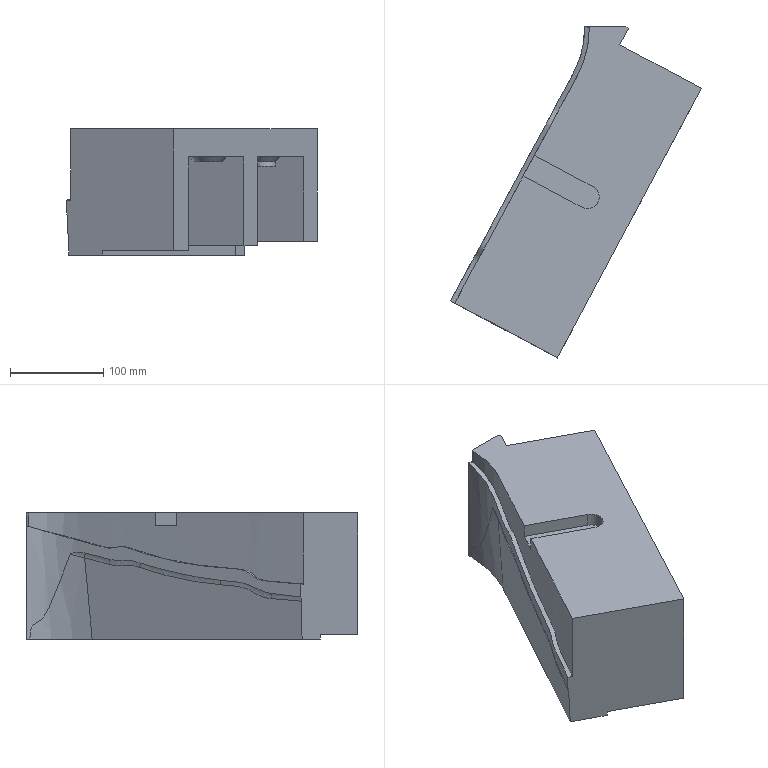Part | NX | features solid 2 | 1 solid | 51 faces | box 268.103 x 355.034 x 135 mm | volume 3330847 mm3 | plane 30 | spline 12 | cone 6 | cylinder 3 | commonest cylinder face diameters 25 x3